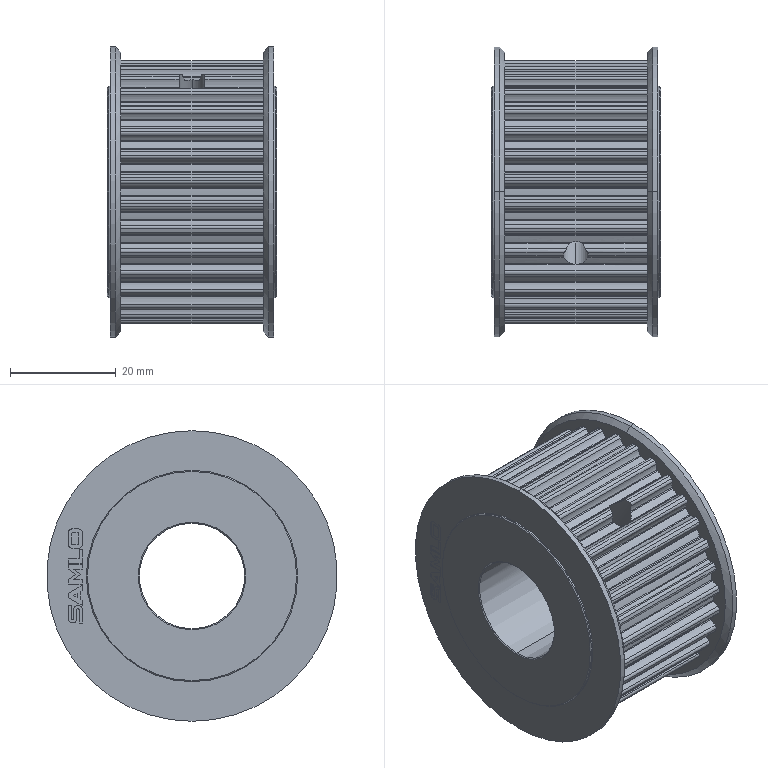Part | SolidWorks | features BaseBody 1, ICE 1 | 1 solid | 401 faces | box 32 x 55 x 55 mm | volume 48801 mm3 | cylinder 331 | plane 58 | cone 12 | commonest cylinder face diameters 1.1 x82 0.5 x81 6.55 x72 46.43 x35 49.97 x33 0.603 x4